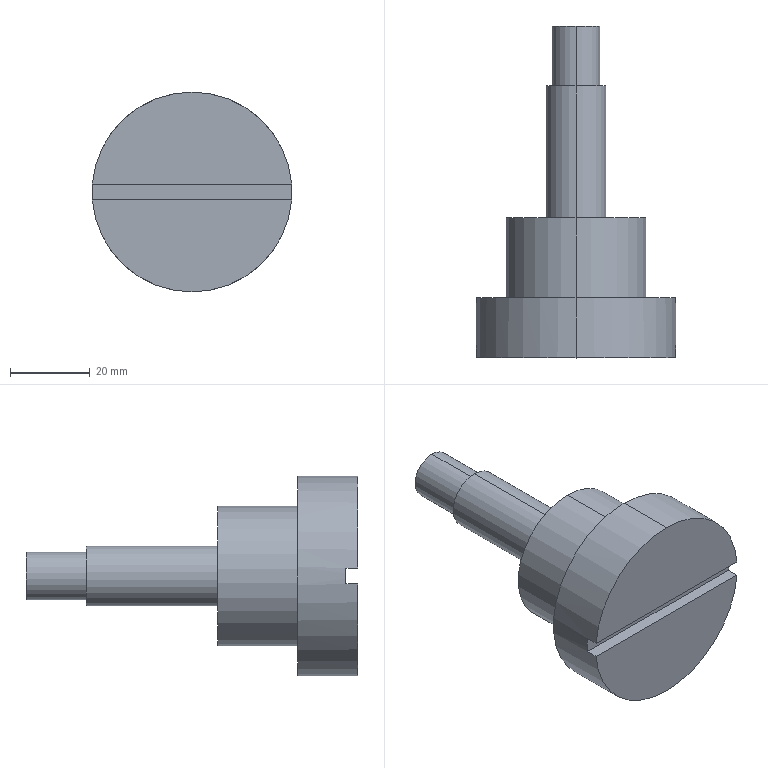Part | STEP file | Large handwheel QY-1-36 | 1 solid | 17 faces | box 50 x 83 x 50 mm | volume 55623 mm3 | plane 9 | cylinder 8 | commonest cylinder face diameters 12 x2 15 x2 35 x2 50 x2
STEP:
#1=CARTESIAN_POINT('',(0.,0.,0.));
#2=DIRECTION('',(0.,0.,1.));
#3=DIRECTION('',(1.,0.,0.));
#4=AXIS2_PLACEMENT_3D('',#1,#2,#3);
#5=CARTESIAN_POINT('',(0.,83.,6.));
#6=VERTEX_POINT('',#5);
#7=CARTESIAN_POINT('',(0.,83.,-6.));
#8=VERTEX_POINT('',#7);
#9=CARTESIAN_POINT('',(0.,83.,0.));
#10=DIRECTION('',(0.,1.,0.));
#11=DIRECTION('',(0.,0.,1.));
#12=AXIS2_PLACEMENT_3D('',#9,#10,#11);
#13=CIRCLE('',#12,6.);
#14=CARTESIAN_POINT('',(0.,83.,0.));
#15=DIRECTION('',(0.,-1.,0.));
#16=DIRECTION('',(0.,0.,-1.));
#17=AXIS2_PLACEMENT_3D('',#14,#15,#16);
#18=CYLINDRICAL_SURFACE('',#17,6.);
#19=CARTESIAN_POINT('',(3.142,0.));
#20=DIRECTION('',(-1.,0.));
#21=VECTOR('',#20,1.);
#22=LINE('',#19,#21);
#23=(GEOMETRIC_REPRESENTATION_CONTEXT(2)PARAMETRIC_REPRESENTATION_CONTEXT()REPRESENTATION_CONTEXT('',''));
#24=DEFINITIONAL_REPRESENTATION('',(#22),#23);
#25=PCURVE('',#18,#24);
#26=CARTESIAN_POINT('',(0.,83.,0.));
#27=DIRECTION('',(0.,1.,0.));
#28=DIRECTION('',(0.,0.,1.));
#29=AXIS2_PLACEMENT_3D('',#26,#27,#28);
#30=PLANE('',#29);
#31=CARTESIAN_POINT('',(0.,0.));
#32=DIRECTION('',(1.,0.));
#33=AXIS2_PLACEMENT_2D('',#31,#32);
#34=CIRCLE('',#33,6.);
#35=(GEOMETRIC_REPRESENTATION_CONTEXT(2)PARAMETRIC_REPRESENTATION_CONTEXT()REPRESENTATION_CONTEXT('',''));
#36=DEFINITIONAL_REPRESENTATION('',(#34),#35);
#37=PCURVE('',#30,#36);
#38=SURFACE_CURVE('',#13,(#25,#37),.PCURVE_S1.);
#39=EDGE_CURVE('',#6,#8,#38,.T.);
#40=ORIENTED_EDGE('',*,*,#39,.F.);
#41=CARTESIAN_POINT('',(0.,68.,6.));
#42=VERTEX_POINT('',#41);
#43=CARTESIAN_POINT('',(0.,83.,6.));
#44=DIRECTION('',(0.,-1.,0.));
#45=VECTOR('',#44,1.);
#46=LINE('',#43,#45);
#47=CARTESIAN_POINT('',(3.142,0.));
#48=DIRECTION('',(0.,1.));
#49=VECTOR('',#48,1.);
#50=LINE('',#47,#49);
#51=(GEOMETRIC_REPRESENTATION_CONTEXT(2)PARAMETRIC_REPRESENTATION_CONTEXT()REPRESENTATION_CONTEXT('',''));
#52=DEFINITIONAL_REPRESENTATION('',(#50),#51);
#53=PCURVE('',#18,#52);
#54=CARTESIAN_POINT('',(0.,83.,0.));
#55=DIRECTION('',(0.,-1.,0.));
#56=DIRECTION('',(0.,0.,-1.));
#57=AXIS2_PLACEMENT_3D('',#54,#55,#56);
#58=CYLINDRICAL_SURFACE('',#57,6.);
#59=CARTESIAN_POINT('',(3.142,0.));
#60=DIRECTION('',(0.,1.));
#61=VECTOR('',#60,1.);
#62=LINE('',#59,#61);
#63=(GEOMETRIC_REPRESENTATION_CONTEXT(2)PARAMETRIC_REPRESENTATION_CONTEXT()REPRESENTATION_CONTEXT('',''));
#64=DEFINITIONAL_REPRESENTATION('',(#62),#63);
#65=PCURVE('',#58,#64);
#66=SURFACE_CURVE('',#46,(#53,#65),.PCURVE_S1.);
#67=EDGE_CURVE('',#6,#42,#66,.T.);
#68=ORIENTED_EDGE('',*,*,#67,.T.);
#69=CARTESIAN_POINT('',(0.,68.,-6.));
#70=VERTEX_POINT('',#69);
#71=CARTESIAN_POINT('',(0.,68.,0.));
#72=DIRECTION('',(0.,1.,0.));
#73=DIRECTION('',(0.,0.,1.));
#74=AXIS2_PLACEMENT_3D('',#71,#72,#73);
#75=CIRCLE('',#74,6.);
#76=CARTESIAN_POINT('',(3.142,15.));
#77=DIRECTION('',(-1.,0.));
#78=VECTOR('',#77,1.);
#79=LINE('',#76,#78);
#80=(GEOMETRIC_REPRESENTATION_CONTEXT(2)PARAMETRIC_REPRESENTATION_CONTEXT()REPRESENTATION_CONTEXT('',''));
#81=DEFINITIONAL_REPRESENTATION('',(#79),#80);
#82=PCURVE('',#18,#81);
#83=CARTESIAN_POINT('',(0.,68.,0.));
#84=DIRECTION('',(0.,1.,0.));
#85=DIRECTION('',(0.,0.,1.));
#86=AXIS2_PLACEMENT_3D('',#83,#84,#85);
#87=PLANE('',#86);
#88=CARTESIAN_POINT('',(0.,0.));
#89=DIRECTION('',(1.,0.));
#90=AXIS2_PLACEMENT_2D('',#88,#89);
#91=CIRCLE('',#90,6.);
#92=(GEOMETRIC_REPRESENTATION_CONTEXT(2)PARAMETRIC_REPRESENTATION_CONTEXT()REPRESENTATION_CONTEXT('',''));
#93=DEFINITIONAL_REPRESENTATION('',(#91),#92);
#94=PCURVE('',#87,#93);
#95=SURFACE_CURVE('',#75,(#82,#94),.PCURVE_S1.);
#96=EDGE_CURVE('',#42,#70,#95,.T.);
#97=ORIENTED_EDGE('',*,*,#96,.T.);
#98=CARTESIAN_POINT('',(0.,83.,-6.));
#99=DIRECTION('',(0.,-1.,0.));
#100=VECTOR('',#99,1.);
#101=LINE('',#98,#100);
#102=CARTESIAN_POINT('',(0.,0.));
#103=DIRECTION('',(0.,1.));
#104=VECTOR('',#103,1.);
#105=LINE('',#102,#104);
#106=(GEOMETRIC_REPRESENTATION_CONTEXT(2)PARAMETRIC_REPRESENTATION_CONTEXT()REPRESENTATION_CONTEXT('',''));
#107=DEFINITIONAL_REPRESENTATION('',(#105),#106);
#108=PCURVE('',#18,#107);
#109=CARTESIAN_POINT('',(6.283,0.));
#110=DIRECTION('',(0.,1.));
#111=VECTOR('',#110,1.);
#112=LINE('',#109,#111);
#113=(GEOMETRIC_REPRESENTATION_CONTEXT(2)PARAMETRIC_REPRESENTATION_CONTEXT()REPRESENTATION_CONTEXT('',''));
#114=DEFINITIONAL_REPRESENTATION('',(#112),#113);
#115=PCURVE('',#58,#114);
#116=SURFACE_CURVE('',#101,(#108,#115),.PCURVE_S1.);
#117=EDGE_CURVE('',#8,#70,#116,.T.);
#118=ORIENTED_EDGE('',*,*,#117,.F.);
#119=EDGE_LOOP('',(#40,#68,#97,#118));
#120=FACE_BOUND('',#119,.T.);
#121=ADVANCED_FACE('',(#120),#18,.T.);
#122=CARTESIAN_POINT('',(0.,68.,7.5));
#123=VERTEX_POINT('',#122);
#124=CARTESIAN_POINT('',(0.,68.,-7.5));
#125=VERTEX_POINT('',#124);
#126=CARTESIAN_POINT('',(0.,68.,0.));
#127=DIRECTION('',(0.,1.,0.));
#128=DIRECTION('',(0.,0.,1.));
#129=AXIS2_PLACEMENT_3D('',#126,#127,#128);
#130=CIRCLE('',#129,7.5);
#131=CARTESIAN_POINT('',(0.,68.,0.));
#132=DIRECTION('',(0.,-1.,0.));
#133=DIRECTION('',(0.,0.,-1.));
#134=AXIS2_PLACEMENT_3D('',#131,#132,#133);
#135=CYLINDRICAL_SURFACE('',#134,7.5);
#136=CARTESIAN_POINT('',(3.142,0.));
#137=DIRECTION('',(-1.,0.));
#138=VECTOR('',#137,1.);
#139=LINE('',#136,#138);
#140=(GEOMETRIC_REPRESENTATION_CONTEXT(2)PARAMETRIC_REPRESENTATION_CONTEXT()REPRESENTATION_CONTEXT('',''));
#141=DEFINITIONAL_REPRESENTATION('',(#139),#140);
#142=PCURVE('',#135,#141);
#143=CARTESIAN_POINT('',(0.,0.));
#144=DIRECTION('',(1.,0.));
#145=AXIS2_PLACEMENT_2D('',#143,#144);
#146=CIRCLE('',#145,7.5);
#147=(GEOMETRIC_REPRESENTATION_CONTEXT(2)PARAMETRIC_REPRESENTATION_CONTEXT()REPRESENTATION_CONTEXT('',''));
#148=DEFINITIONAL_REPRESENTATION('',(#146),#147);
#149=PCURVE('',#87,#148);
#150=SURFACE_CURVE('',#130,(#142,#149),.PCURVE_S1.);
#151=EDGE_CURVE('',#123,#125,#150,.T.);
#152=ORIENTED_EDGE('',*,*,#151,.F.);
#153=CARTESIAN_POINT('',(0.,35.,7.5));
#154=VERTEX_POINT('',#153);
#155=CARTESIAN_POINT('',(0.,68.,7.5));
#156=DIRECTION('',(0.,-1.,0.));
#157=VECTOR('',#156,1.);
#158=LINE('',#155,#157);
#159=CARTESIAN_POINT('',(3.142,0.));
#160=DIRECTION('',(0.,1.));
#161=VECTOR('',#160,1.);
#162=LINE('',#159,#161);
#163=(GEOMETRIC_REPRESENTATION_CONTEXT(2)PARAMETRIC_REPRESENTATION_CONTEXT()REPRESENTATION_CONTEXT('',''));
#164=DEFINITIONAL_REPRESENTATION('',(#162),#163);
#165=PCURVE('',#135,#164);
#166=CARTESIAN_POINT('',(0.,68.,0.));
#167=DIRECTION('',(0.,-1.,0.));
#168=DIRECTION('',(0.,0.,-1.));
#169=AXIS2_PLACEMENT_3D('',#166,#167,#168);
#170=CYLINDRICAL_SURFACE('',#169,7.5);
#171=CARTESIAN_POINT('',(3.142,0.));
#172=DIRECTION('',(0.,1.));
#173=VECTOR('',#172,1.);
#174=LINE('',#171,#173);
#175=(GEOMETRIC_REPRESENTATION_CONTEXT(2)PARAMETRIC_REPRESENTATION_CONTEXT()REPRESENTATION_CONTEXT('',''));
#176=DEFINITIONAL_REPRESENTATION('',(#174),#175);
#177=PCURVE('',#170,#176);
#178=SURFACE_CURVE('',#158,(#165,#177),.PCURVE_S1.);
#179=EDGE_CURVE('',#123,#154,#178,.T.);
#180=ORIENTED_EDGE('',*,*,#179,.T.);
#181=CARTESIAN_POINT('',(0.,35.,-7.5));
#182=VERTEX_POINT('',#181);
#183=CARTESIAN_POINT('',(0.,35.,0.));
#184=DIRECTION('',(0.,1.,0.));
#185=DIRECTION('',(0.,0.,1.));
#186=AXIS2_PLACEMENT_3D('',#183,#184,#185);
#187=CIRCLE('',#186,7.5);
#188=CARTESIAN_POINT('',(3.142,33.));
#189=DIRECTION('',(-1.,0.));
#190=VECTOR('',#189,1.);
#191=LINE('',#188,#190);
#192=(GEOMETRIC_REPRESENTATION_CONTEXT(2)PARAMETRIC_REPRESENTATION_CONTEXT()REPRESENTATION_CONTEXT('',''));
#193=DEFINITIONAL_REPRESENTATION('',(#191),#192);
#194=PCURVE('',#135,#193);
#195=CARTESIAN_POINT('',(0.,35.,0.));
#196=DIRECTION('',(0.,1.,0.));
#197=DIRECTION('',(0.,0.,1.));
#198=AXIS2_PLACEMENT_3D('',#195,#196,#197);
#199=PLANE('',#198);
#200=CARTESIAN_POINT('',(0.,0.));
#201=DIRECTION('',(1.,0.));
#202=AXIS2_PLACEMENT_2D('',#200,#201);
#203=CIRCLE('',#202,7.5);
#204=(GEOMETRIC_REPRESENTATION_CONTEXT(2)PARAMETRIC_REPRESENTATION_CONTEXT()REPRESENTATION_CONTEXT('',''));
#205=DEFINITIONAL_REPRESENTATION('',(#203),#204);
#206=PCURVE('',#199,#205);
#207=SURFACE_CURVE('',#187,(#194,#206),.PCURVE_S1.);
#208=EDGE_CURVE('',#154,#182,#207,.T.);
#209=ORIENTED_EDGE('',*,*,#208,.T.);
#210=CARTESIAN_POINT('',(0.,68.,-7.5));
#211=DIRECTION('',(0.,-1.,0.));
#212=VECTOR('',#211,1.);
#213=LINE('',#210,#212);
#214=CARTESIAN_POINT('',(0.,0.));
#215=DIRECTION('',(0.,1.));
#216=VECTOR('',#215,1.);
#217=LINE('',#214,#216);
#218=(GEOMETRIC_REPRESENTATION_CONTEXT(2)PARAMETRIC_REPRESENTATION_CONTEXT()REPRESENTATION_CONTEXT('',''));
#219=DEFINITIONAL_REPRESENTATION('',(#217),#218);
#220=PCURVE('',#135,#219);
#221=CARTESIAN_POINT('',(6.283,0.));
#222=DIRECTION('',(0.,1.));
#223=VECTOR('',#222,1.);
#224=LINE('',#221,#223);
#225=(GEOMETRIC_REPRESENTATION_CONTEXT(2)PARAMETRIC_REPRESENTATION_CONTEXT()REPRESENTATION_CONTEXT('',''));
#226=DEFINITIONAL_REPRESENTATION('',(#224),#225);
#227=PCURVE('',#170,#226);
#228=SURFACE_CURVE('',#213,(#220,#227),.PCURVE_S1.);
#229=EDGE_CURVE('',#125,#182,#228,.T.);
#230=ORIENTED_EDGE('',*,*,#229,.F.);
#231=EDGE_LOOP('',(#152,#180,#209,#230));
#232=FACE_BOUND('',#231,.T.);
#233=ADVANCED_FACE('',(#232),#135,.T.);
#234=CARTESIAN_POINT('',(0.,35.,17.5));
#235=VERTEX_POINT('',#234);
#236=CARTESIAN_POINT('',(0.,35.,-17.5));
#237=VERTEX_POINT('',#236);
#238=CARTESIAN_POINT('',(0.,35.,0.));
#239=DIRECTION('',(0.,1.,0.));
#240=DIRECTION('',(0.,0.,1.));
#241=AXIS2_PLACEMENT_3D('',#238,#239,#240);
#242=CIRCLE('',#241,17.5);
#243=CARTESIAN_POINT('',(0.,35.,0.));
#244=DIRECTION('',(0.,-1.,0.));
#245=DIRECTION('',(0.,0.,-1.));
#246=AXIS2_PLACEMENT_3D('',#243,#244,#245);
#247=CYLINDRICAL_SURFACE('',#246,17.5);
#248=CARTESIAN_POINT('',(3.142,0.));
#249=DIRECTION('',(-1.,0.));
#250=VECTOR('',#249,1.);
#251=LINE('',#248,#250);
#252=(GEOMETRIC_REPRESENTATION_CONTEXT(2)PARAMETRIC_REPRESENTATION_CONTEXT()REPRESENTATION_CONTEXT('',''));
#253=DEFINITIONAL_REPRESENTATION('',(#251),#252);
#254=PCURVE('',#247,#253);
#255=CARTESIAN_POINT('',(0.,0.));
#256=DIRECTION('',(1.,0.));
#257=AXIS2_PLACEMENT_2D('',#255,#256);
#258=CIRCLE('',#257,17.5);
#259=(GEOMETRIC_REPRESENTATION_CONTEXT(2)PARAMETRIC_REPRESENTATION_CONTEXT()REPRESENTATION_CONTEXT('',''));
#260=DEFINITIONAL_REPRESENTATION('',(#258),#259);
#261=PCURVE('',#199,#260);
#262=SURFACE_CURVE('',#242,(#254,#261),.PCURVE_S1.);
#263=EDGE_CURVE('',#235,#237,#262,.T.);
#264=ORIENTED_EDGE('',*,*,#263,.F.);
#265=CARTESIAN_POINT('',(0.,15.,17.5));
#266=VERTEX_POINT('',#265);
#267=CARTESIAN_POINT('',(0.,35.,17.5));
#268=DIRECTION('',(0.,-1.,0.));
#269=VECTOR('',#268,1.);
#270=LINE('',#267,#269);
#271=CARTESIAN_POINT('',(3.142,0.));
#272=DIRECTION('',(0.,1.));
#273=VECTOR('',#272,1.);
#274=LINE('',#271,#273);
#275=(GEOMETRIC_REPRESENTATION_CONTEXT(2)PARAMETRIC_REPRESENTATION_CONTEXT()REPRESENTATION_CONTEXT('',''));
#276=DEFINITIONAL_REPRESENTATION('',(#274),#275);
#277=PCURVE('',#247,#276);
#278=CARTESIAN_POINT('',(0.,35.,0.));
#279=DIRECTION('',(0.,-1.,0.));
#280=DIRECTION('',(0.,0.,-1.));
#281=AXIS2_PLACEMENT_3D('',#278,#279,#280);
#282=CYLINDRICAL_SURFACE('',#281,17.5);
#283=CARTESIAN_POINT('',(3.142,0.));
#284=DIRECTION('',(0.,1.));
#285=VECTOR('',#284,1.);
#286=LINE('',#283,#285);
#287=(GEOMETRIC_REPRESENTATION_CONTEXT(2)PARAMETRIC_REPRESENTATION_CONTEXT()REPRESENTATION_CONTEXT('',''));
#288=DEFINITIONAL_REPRESENTATION('',(#286),#287);
#289=PCURVE('',#282,#288);
#290=SURFACE_CURVE('',#270,(#277,#289),.PCURVE_S1.);
#291=EDGE_CURVE('',#235,#266,#290,.T.);
#292=ORIENTED_EDGE('',*,*,#291,.T.);
#293=CARTESIAN_POINT('',(0.,15.,-17.5));
#294=VERTEX_POINT('',#293);
#295=CARTESIAN_POINT('',(0.,15.,0.));
#296=DIRECTION('',(0.,1.,0.));
#297=DIRECTION('',(0.,0.,1.));
#298=AXIS2_PLACEMENT_3D('',#295,#296,#297);
#299=CIRCLE('',#298,17.5);
#300=CARTESIAN_POINT('',(3.142,20.));
#301=DIRECTION('',(-1.,0.));
#302=VECTOR('',#301,1.);
#303=LINE('',#300,#302);
#304=(GEOMETRIC_REPRESENTATION_CONTEXT(2)PARAMETRIC_REPRESENTATION_CONTEXT()REPRESENTATION_CONTEXT('',''));
#305=DEFINITIONAL_REPRESENTATION('',(#303),#304);
#306=PCURVE('',#247,#305);
#307=CARTESIAN_POINT('',(0.,15.,0.));
#308=DIRECTION('',(0.,1.,0.));
#309=DIRECTION('',(0.,0.,1.));
#310=AXIS2_PLACEMENT_3D('',#307,#308,#309);
#311=PLANE('',#310);
#312=CARTESIAN_POINT('',(0.,0.));
#313=DIRECTION('',(1.,0.));
#314=AXIS2_PLACEMENT_2D('',#312,#313);
#315=CIRCLE('',#314,17.5);
#316=(GEOMETRIC_REPRESENTATION_CONTEXT(2)PARAMETRIC_REPRESENTATION_CONTEXT()REPRESENTATION_CONTEXT('',''));
#317=DEFINITIONAL_REPRESENTATION('',(#315),#316);
#318=PCURVE('',#311,#317);
#319=SURFACE_CURVE('',#299,(#306,#318),.PCURVE_S1.);
#320=EDGE_CURVE('',#266,#294,#319,.T.);
#321=ORIENTED_EDGE('',*,*,#320,.T.);
#322=CARTESIAN_POINT('',(0.,35.,-17.5));
#323=DIRECTION('',(0.,-1.,0.));
#324=VECTOR('',#323,1.);
#325=LINE('',#322,#324);
#326=CARTESIAN_POINT('',(0.,0.));
#327=DIRECTION('',(0.,1.));
#328=VECTOR('',#327,1.);
#329=LINE('',#326,#328);
#330=(GEOMETRIC_REPRESENTATION_CONTEXT(2)PARAMETRIC_REPRESENTATION_CONTEXT()REPRESENTATION_CONTEXT('',''));
#331=DEFINITIONAL_REPRESENTATION('',(#329),#330);
#332=PCURVE('',#247,#331);
#333=CARTESIAN_POINT('',(6.283,0.));
#334=DIRECTION('',(0.,1.));
#335=VECTOR('',#334,1.);
#336=LINE('',#333,#335);
#337=(GEOMETRIC_REPRESENTATION_CONTEXT(2)PARAMETRIC_REPRESENTATION_CONTEXT()REPRESENTATION_CONTEXT('',''));
#338=DEFINITIONAL_REPRESENTATION('',(#336),#337);
#339=PCURVE('',#282,#338);
#340=SURFACE_CURVE('',#325,(#332,#339),.PCURVE_S1.);
#341=EDGE_CURVE('',#237,#294,#340,.T.);
#342=ORIENTED_EDGE('',*,*,#341,.F.);
#343=EDGE_LOOP('',(#264,#292,#321,#342));
#344=FACE_BOUND('',#343,.T.);
#345=ADVANCED_FACE('',(#344),#247,.T.);
#346=CARTESIAN_POINT('',(0.,15.,25.));
#347=VERTEX_POINT('',#346);
#348=CARTESIAN_POINT('',(0.,15.,-25.));
#349=VERTEX_POINT('',#348);
#350=CARTESIAN_POINT('',(0.,15.,0.));
#351=DIRECTION('',(0.,1.,0.));
#352=DIRECTION('',(0.,0.,1.));
#353=AXIS2_PLACEMENT_3D('',#350,#351,#352);
#354=CIRCLE('',#353,25.);
#355=CARTESIAN_POINT('',(0.,15.,0.));
#356=DIRECTION('',(0.,-1.,0.));
#357=DIRECTION('',(0.,0.,-1.));
#358=AXIS2_PLACEMENT_3D('',#355,#356,#357);
#359=CYLINDRICAL_SURFACE('',#358,25.);
#360=CARTESIAN_POINT('',(3.142,0.));
#361=DIRECTION('',(-1.,0.));
#362=VECTOR('',#361,1.);
#363=LINE('',#360,#362);
#364=(GEOMETRIC_REPRESENTATION_CONTEXT(2)PARAMETRIC_REPRESENTATION_CONTEXT()REPRESENTATION_CONTEXT('',''));
#365=DEFINITIONAL_REPRESENTATION('',(#363),#364);
#366=PCURVE('',#359,#365);
#367=CARTESIAN_POINT('',(0.,0.));
#368=DIRECTION('',(1.,0.));
#369=AXIS2_PLACEMENT_2D('',#367,#368);
#370=CIRCLE('',#369,25.);
#371=(GEOMETRIC_REPRESENTATION_CONTEXT(2)PARAMETRIC_REPRESENTATION_CONTEXT()REPRESENTATION_CONTEXT('',''));
#372=DEFINITIONAL_REPRESENTATION('',(#370),#371);
#373=PCURVE('',#311,#372);
#374=SURFACE_CURVE('',#354,(#366,#373),.PCURVE_S1.);
#375=EDGE_CURVE('',#347,#349,#374,.T.);
#376=ORIENTED_EDGE('',*,*,#375,.F.);
#377=CARTESIAN_POINT('',(0.,0.,25.));
#378=VERTEX_POINT('',#377);
#379=CARTESIAN_POINT('',(0.,15.,25.));
#380=DIRECTION('',(0.,-1.,0.));
#381=VECTOR('',#380,1.);
#382=LINE('',#379,#381);
#383=CARTESIAN_POINT('',(3.142,0.));
#384=DIRECTION('',(0.,1.));
#385=VECTOR('',#384,1.);
#386=LINE('',#383,#385);
#387=(GEOMETRIC_REPRESENTATION_CONTEXT(2)PARAMETRIC_REPRESENTATION_CONTEXT()REPRESENTATION_CONTEXT('',''));
#388=DEFINITIONAL_REPRESENTATION('',(#386),#387);
#389=PCURVE('',#359,#388);
#390=CARTESIAN_POINT('',(0.,15.,0.));
#391=DIRECTION('',(0.,-1.,0.));
#392=DIRECTION('',(0.,0.,-1.));
#393=AXIS2_PLACEMENT_3D('',#390,#391,#392);
#394=CYLINDRICAL_SURFACE('',#393,25.);
#395=CARTESIAN_POINT('',(3.142,0.));
#396=DIRECTION('',(0.,1.));
#397=VECTOR('',#396,1.);
#398=LINE('',#395,#397);
#399=(GEOMETRIC_REPRESENTATION_CONTEXT(2)PARAMETRIC_REPRESENTATION_CONTEXT()REPRESENTATION_CONTEXT('',''));
#400=DEFINITIONAL_REPRESENTATION('',(#398),#399);
#401=PCURVE('',#394,#400);
#402=SURFACE_CURVE('',#382,(#389,#401),.PCURVE_S1.);
#403=EDGE_CURVE('',#347,#378,#402,.T.);
#404=ORIENTED_EDGE('',*,*,#403,.T.);
#405=CARTESIAN_POINT('',(24.92,0.,2.));
#406=VERTEX_POINT('',#405);
#407=CARTESIAN_POINT('',(0.,0.,0.));
#408=DIRECTION('',(0.,1.,0.));
#409=DIRECTION('',(0.,0.,1.));
#410=AXIS2_PLACEMENT_3D('',#407,#408,#409);
#411=CIRCLE('',#410,25.);
#412=CARTESIAN_POINT('',(3.142,15.));
#413=DIRECTION('',(-1.,0.));
#414=VECTOR('',#413,1.);
#415=LINE('',#412,#414);
#416=(GEOMETRIC_REPRESENTATION_CONTEXT(2)PARAMETRIC_REPRESENTATION_CONTEXT()REPRESENTATION_CONTEXT('',''));
#417=DEFINITIONAL_REPRESENTATION('',(#415),#416);
#418=PCURVE('',#359,#417);
#419=CARTESIAN_POINT('',(0.,0.,0.));
#420=DIRECTION('',(0.,1.,0.));
#421=DIRECTION('',(0.,0.,1.));
#422=AXIS2_PLACEMENT_3D('',#419,#420,#421);
#423=PLANE('',#422);
#424=CARTESIAN_POINT('',(0.,0.));
#425=DIRECTION('',(1.,0.));
#426=AXIS2_PLACEMENT_2D('',#424,#425);
#427=CIRCLE('',#426,25.);
#428=(GEOMETRIC_REPRESENTATION_CONTEXT(2)PARAMETRIC_REPRESENTATION_CONTEXT()REPRESENTATION_CONTEXT('',''));
#429=DEFINITIONAL_REPRESENTATION('',(#427),#428);
#430=PCURVE('',#423,#429);
#431=SURFACE_CURVE('',#411,(#418,#430),.PCURVE_S1.);
#432=EDGE_CURVE('',#378,#406,#431,.T.);
#433=ORIENTED_EDGE('',*,*,#432,.T.);
#434=CARTESIAN_POINT('',(24.92,3.,2.));
#435=VERTEX_POINT('',#434);
#436=CARTESIAN_POINT('',(24.92,15.,2.));
#437=DIRECTION('',(0.,1.,0.));
#438=VECTOR('',#437,1.);
#439=LINE('',#436,#438);
#440=CARTESIAN_POINT('',(1.651,0.));
#441=DIRECTION('',(0.,-1.));
#442=VECTOR('',#441,1.);
#443=LINE('',#440,#442);
#444=(GEOMETRIC_REPRESENTATION_CONTEXT(2)PARAMETRIC_REPRESENTATION_CONTEXT()REPRESENTATION_CONTEXT('',''));
#445=DEFINITIONAL_REPRESENTATION('',(#443),#444);
#446=PCURVE('',#359,#445);
#447=CARTESIAN_POINT('',(-71.5,3.,2.));
#448=DIRECTION('',(0.,0.,1.));
#449=DIRECTION('',(1.,0.,0.));
#450=AXIS2_PLACEMENT_3D('',#447,#448,#449);
#451=PLANE('',#450);
#452=CARTESIAN_POINT('',(96.42,12.));
#453=DIRECTION('',(0.,1.));
#454=VECTOR('',#453,1.);
#455=LINE('',#452,#454);
#456=(GEOMETRIC_REPRESENTATION_CONTEXT(2)PARAMETRIC_REPRESENTATION_CONTEXT()REPRESENTATION_CONTEXT('',''));
#457=DEFINITIONAL_REPRESENTATION('',(#455),#456);
#458=PCURVE('',#451,#457);
#459=SURFACE_CURVE('',#439,(#446,#458),.PCURVE_S1.);
#460=EDGE_CURVE('',#406,#435,#459,.T.);
#461=ORIENTED_EDGE('',*,*,#460,.T.);
#462=CARTESIAN_POINT('',(24.92,3.,-2.));
#463=VERTEX_POINT('',#462);
#464=CARTESIAN_POINT('',(0.,3.,0.));
#465=DIRECTION('',(0.,1.,0.));
#466=DIRECTION('',(0.,0.,1.));
#467=AXIS2_PLACEMENT_3D('',#464,#465,#466);
#468=CIRCLE('',#467,25.);
#469=CARTESIAN_POINT('',(3.142,12.));
#470=DIRECTION('',(-1.,0.));
#471=VECTOR('',#470,1.);
#472=LINE('',#469,#471);
#473=(GEOMETRIC_REPRESENTATION_CONTEXT(2)PARAMETRIC_REPRESENTATION_CONTEXT()REPRESENTATION_CONTEXT('',''));
#474=DEFINITIONAL_REPRESENTATION('',(#472),#473);
#475=PCURVE('',#359,#474);
#476=CARTESIAN_POINT('',(-71.5,3.,2.));
#477=DIRECTION('',(0.,1.,0.));
#478=DIRECTION('',(0.,0.,1.));
#479=AXIS2_PLACEMENT_3D('',#476,#477,#478);
#480=PLANE('',#479);
#481=CARTESIAN_POINT('',(-2.,71.5));
#482=DIRECTION('',(1.,0.));
#483=AXIS2_PLACEMENT_2D('',#481,#482);
#484=CIRCLE('',#483,25.);
#485=(GEOMETRIC_REPRESENTATION_CONTEXT(2)PARAMETRIC_REPRESENTATION_CONTEXT()REPRESENTATION_CONTEXT('',''));
#486=DEFINITIONAL_REPRESENTATION('',(#484),#485);
#487=PCURVE('',#480,#486);
#488=SURFACE_CURVE('',#468,(#475,#487),.PCURVE_S1.);
#489=EDGE_CURVE('',#435,#463,#488,.T.);
#490=ORIENTED_EDGE('',*,*,#489,.T.);
#491=CARTESIAN_POINT('',(24.92,0.,-2.));
#492=VERTEX_POINT('',#491);
#493=CARTESIAN_POINT('',(24.92,15.,-2.));
#494=DIRECTION('',(0.,-1.,0.));
#495=VECTOR('',#494,1.);
#496=LINE('',#493,#495);
#497=CARTESIAN_POINT('',(1.491,0.));
#498=DIRECTION('',(0.,1.));
#499=VECTOR('',#498,1.);
#500=LINE('',#497,#499);
#501=(GEOMETRIC_REPRESENTATION_CONTEXT(2)PARAMETRIC_REPRESENTATION_CONTEXT()REPRESENTATION_CONTEXT('',''));
#502=DEFINITIONAL_REPRESENTATION('',(#500),#501);
#503=PCURVE('',#359,#502);
#504=CARTESIAN_POINT('',(-71.5,3.,-2.));
#505=DIRECTION('',(0.,0.,-1.));
#506=DIRECTION('',(-1.,0.,0.));
#507=AXIS2_PLACEMENT_3D('',#504,#505,#506);
#508=PLANE('',#507);
#509=CARTESIAN_POINT('',(-96.42,12.));
#510=DIRECTION('',(0.,-1.));
#511=VECTOR('',#510,1.);
#512=LINE('',#509,#511);
#513=(GEOMETRIC_REPRESENTATION_CONTEXT(2)PARAMETRIC_REPRESENTATION_CONTEXT()REPRESENTATION_CONTEXT('',''));
#514=DEFINITIONAL_REPRESENTATION('',(#512),#513);
#515=PCURVE('',#508,#514);
#516=SURFACE_CURVE('',#496,(#503,#515),.PCURVE_S1.);
#517=EDGE_CURVE('',#463,#492,#516,.T.);
#518=ORIENTED_EDGE('',*,*,#517,.T.);
#519=CARTESIAN_POINT('',(0.,0.,-25.));
#520=VERTEX_POINT('',#519);
#521=CARTESIAN_POINT('',(0.,0.,0.));
#522=DIRECTION('',(0.,1.,0.));
#523=DIRECTION('',(0.,0.,1.));
#524=AXIS2_PLACEMENT_3D('',#521,#522,#523);
#525=CIRCLE('',#524,25.);
#526=CARTESIAN_POINT('',(3.142,15.));
#527=DIRECTION('',(-1.,0.));
#528=VECTOR('',#527,1.);
#529=LINE('',#526,#528);
#530=(GEOMETRIC_REPRESENTATION_CONTEXT(2)PARAMETRIC_REPRESENTATION_CONTEXT()REPRESENTATION_CONTEXT('',''));
#531=DEFINITIONAL_REPRESENTATION('',(#529),#530);
#532=PCURVE('',#359,#531);
#533=CARTESIAN_POINT('',(0.,0.,0.));
#534=DIRECTION('',(0.,1.,0.));
#535=DIRECTION('',(0.,0.,1.));
#536=AXIS2_PLACEMENT_3D('',#533,#534,#535);
#537=PLANE('',#536);
#538=CARTESIAN_POINT('',(0.,0.));
#539=DIRECTION('',(1.,0.));
#540=AXIS2_PLACEMENT_2D('',#538,#539);
#541=CIRCLE('',#540,25.);
#542=(GEOMETRIC_REPRESENTATION_CONTEXT(2)PARAMETRIC_REPRESENTATION_CONTEXT()REPRESENTATION_CONTEXT('',''));
#543=DEFINITIONAL_REPRESENTATION('',(#541),#542);
#544=PCURVE('',#537,#543);
#545=SURFACE_CURVE('',#525,(#532,#544),.PCURVE_S1.);
#546=EDGE_CURVE('',#492,#520,#545,.T.);
#547=ORIENTED_EDGE('',*,*,#546,.T.);
#548=CARTESIAN_POINT('',(0.,15.,-25.));
#549=DIRECTION('',(0.,-1.,0.));
#550=VECTOR('',#549,1.);
#551=LINE('',#548,#550);
#552=CARTESIAN_POINT('',(0.,0.));
#553=DIRECTION('',(0.,1.));
#554=VECTOR('',#553,1.);
#555=LINE('',#552,#554);
#556=(GEOMETRIC_REPRESENTATION_CONTEXT(2)PARAMETRIC_REPRESENTATION_CONTEXT()REPRESENTATION_CONTEXT('',''));
#557=DEFINITIONAL_REPRESENTATION('',(#555),#556);
#558=PCURVE('',#359,#557);
#559=CARTESIAN_POINT('',(6.283,0.));
#560=DIRECTION('',(0.,1.));
#561=VECTOR('',#560,1.);
#562=LINE('',#559,#561);
#563=(GEOMETRIC_REPRESENTATION_CONTEXT(2)PARAMETRIC_REPRESENTATION_CONTEXT()REPRESENTATION_CONTEXT('',''));
#564=DEFINITIONAL_REPRESENTATION('',(#562),#563);
#565=PCURVE('',#394,#564);
#566=SURFACE_CURVE('',#551,(#558,#565),.PCURVE_S1.);
#567=EDGE_CURVE('',#349,#520,#566,.T.);
#568=ORIENTED_EDGE('',*,*,#567,.F.);
#569=EDGE_LOOP('',(#376,#404,#433,#461,#490,#518,#547,#568));
#570=FACE_BOUND('',#569,.T.);
#571=ADVANCED_FACE('',(#570),#359,.T.);
#572=ORIENTED_EDGE('',*,*,#546,.F.);
#573=CARTESIAN_POINT('',(-24.92,0.,-2.));
#574=VERTEX_POINT('',#573);
#575=CARTESIAN_POINT('',(0.,0.,-2.));
#576=DIRECTION('',(-1.,0.,0.));
#577=VECTOR('',#576,1.);
#578=LINE('',#575,#577);
#579=CARTESIAN_POINT('',(-2.,0.));
#580=DIRECTION('',(0.,-1.));
#581=VECTOR('',#580,1.);
#582=LINE('',#579,#581);
#583=(GEOMETRIC_REPRESENTATION_CONTEXT(2)PARAMETRIC_REPRESENTATION_CONTEXT()REPRESENTATION_CONTEXT('',''));
#584=DEFINITIONAL_REPRESENTATION('',(#582),#583);
#585=PCURVE('',#537,#584);
#586=CARTESIAN_POINT('',(-71.5,-3.));
#587=DIRECTION('',(1.,0.));
#588=VECTOR('',#587,1.);
#589=LINE('',#586,#588);
#590=(GEOMETRIC_REPRESENTATION_CONTEXT(2)PARAMETRIC_REPRESENTATION_CONTEXT()REPRESENTATION_CONTEXT('',''));
#591=DEFINITIONAL_REPRESENTATION('',(#589),#590);
#592=PCURVE('',#508,#591);
#593=SURFACE_CURVE('',#578,(#585,#592),.PCURVE_S1.);
#594=EDGE_CURVE('',#492,#574,#593,.T.);
#595=ORIENTED_EDGE('',*,*,#594,.T.);
#596=CARTESIAN_POINT('',(0.,0.,0.));
#597=DIRECTION('',(0.,1.,0.));
#598=DIRECTION('',(0.,0.,1.));
#599=AXIS2_PLACEMENT_3D('',#596,#597,#598);
#600=CIRCLE('',#599,25.);
#601=CARTESIAN_POINT('',(0.,0.));
#602=DIRECTION('',(1.,0.));
#603=AXIS2_PLACEMENT_2D('',#601,#602);
#604=CIRCLE('',#603,25.);
#605=(GEOMETRIC_REPRESENTATION_CONTEXT(2)PARAMETRIC_REPRESENTATION_CONTEXT()REPRESENTATION_CONTEXT('',''));
#606=DEFINITIONAL_REPRESENTATION('',(#604),#605);
#607=PCURVE('',#537,#606);
#608=CARTESIAN_POINT('',(9.425,15.));
#609=DIRECTION('',(-1.,0.));
#610=VECTOR('',#609,1.);
#611=LINE('',#608,#610);
#612=(GEOMETRIC_REPRESENTATION_CONTEXT(2)PARAMETRIC_REPRESENTATION_CONTEXT()REPRESENTATION_CONTEXT('',''));
#613=DEFINITIONAL_REPRESENTATION('',(#611),#612);
#614=PCURVE('',#394,#613);
#615=SURFACE_CURVE('',#600,(#607,#614),.PCURVE_S1.);
#616=EDGE_CURVE('',#520,#574,#615,.T.);
#617=ORIENTED_EDGE('',*,*,#616,.F.);
#618=EDGE_LOOP('',(#572,#595,#617));
#619=FACE_BOUND('',#618,.T.);
#620=ADVANCED_FACE('',(#619),#537,.F.);
#621=ORIENTED_EDGE('',*,*,#403,.F.);
#622=CARTESIAN_POINT('',(0.,15.,0.));
#623=DIRECTION('',(0.,1.,0.));
#624=DIRECTION('',(0.,0.,1.));
#625=AXIS2_PLACEMENT_3D('',#622,#623,#624);
#626=CIRCLE('',#625,25.);
#627=CARTESIAN_POINT('',(9.425,0.));
#628=DIRECTION('',(-1.,0.));
#629=VECTOR('',#628,1.);
#630=LINE('',#627,#629);
#631=(GEOMETRIC_REPRESENTATION_CONTEXT(2)PARAMETRIC_REPRESENTATION_CONTEXT()REPRESENTATION_CONTEXT('',''));
#632=DEFINITIONAL_REPRESENTATION('',(#630),#631);
#633=PCURVE('',#394,#632);
#634=CARTESIAN_POINT('',(0.,0.));
#635=DIRECTION('',(1.,0.));
#636=AXIS2_PLACEMENT_2D('',#634,#635);
#637=CIRCLE('',#636,25.);
#638=(GEOMETRIC_REPRESENTATION_CONTEXT(2)PARAMETRIC_REPRESENTATION_CONTEXT()REPRESENTATION_CONTEXT('',''));
#639=DEFINITIONAL_REPRESENTATION('',(#637),#638);
#640=PCURVE('',#311,#639);
#641=SURFACE_CURVE('',#626,(#633,#640),.PCURVE_S1.);
#642=EDGE_CURVE('',#349,#347,#641,.T.);
#643=ORIENTED_EDGE('',*,*,#642,.F.);
#644=ORIENTED_EDGE('',*,*,#567,.T.);
#645=ORIENTED_EDGE('',*,*,#616,.T.);
#646=CARTESIAN_POINT('',(-24.92,3.,-2.));
#647=VERTEX_POINT('',#646);
#648=CARTESIAN_POINT('',(-24.92,15.,-2.));
#649=DIRECTION('',(0.,1.,0.));
#650=VECTOR('',#649,1.);
#651=LINE('',#648,#650);
#652=CARTESIAN_POINT('',(4.792,0.));
#653=DIRECTION('',(0.,-1.));
#654=VECTOR('',#653,1.);
#655=LINE('',#652,#654);
#656=(GEOMETRIC_REPRESENTATION_CONTEXT(2)PARAMETRIC_REPRESENTATION_CONTEXT()REPRESENTATION_CONTEXT('',''));
#657=DEFINITIONAL_REPRESENTATION('',(#655),#656);
#658=PCURVE('',#394,#657);
#659=CARTESIAN_POINT('',(-46.58,12.));
#660=DIRECTION('',(0.,1.));
#661=VECTOR('',#660,1.);
#662=LINE('',#659,#661);
#663=(GEOMETRIC_REPRESENTATION_CONTEXT(2)PARAMETRIC_REPRESENTATION_CONTEXT()REPRESENTATION_CONTEXT('',''));
#664=DEFINITIONAL_REPRESENTATION('',(#662),#663);
#665=PCURVE('',#508,#664);
#666=SURFACE_CURVE('',#651,(#658,#665),.PCURVE_S1.);
#667=EDGE_CURVE('',#574,#647,#666,.T.);
#668=ORIENTED_EDGE('',*,*,#667,.T.);
#669=CARTESIAN_POINT('',(-24.92,3.,2.));
#670=VERTEX_POINT('',#669);
#671=CARTESIAN_POINT('',(0.,3.,0.));
#672=DIRECTION('',(0.,1.,0.));
#673=DIRECTION('',(0.,0.,1.));
#674=AXIS2_PLACEMENT_3D('',#671,#672,#673);
#675=CIRCLE('',#674,25.);
#676=CARTESIAN_POINT('',(9.425,12.));
#677=DIRECTION('',(-1.,0.));
#678=VECTOR('',#677,1.);
#679=LINE('',#676,#678);
#680=(GEOMETRIC_REPRESENTATION_CONTEXT(2)PARAMETRIC_REPRESENTATION_CONTEXT()REPRESENTATION_CONTEXT('',''));
#681=DEFINITIONAL_REPRESENTATION('',(#679),#680);
#682=PCURVE('',#394,#681);
#683=CARTESIAN_POINT('',(-2.,71.5));
#684=DIRECTION('',(1.,0.));
#685=AXIS2_PLACEMENT_2D('',#683,#684);
#686=CIRCLE('',#685,25.);
#687=(GEOMETRIC_REPRESENTATION_CONTEXT(2)PARAMETRIC_REPRESENTATION_CONTEXT()REPRESENTATION_CONTEXT('',''));
#688=DEFINITIONAL_REPRESENTATION('',(#686),#687);
#689=PCURVE('',#480,#688);
#690=SURFACE_CURVE('',#675,(#682,#689),.PCURVE_S1.);
#691=EDGE_CURVE('',#647,#670,#690,.T.);
#692=ORIENTED_EDGE('',*,*,#691,.T.);
#693=CARTESIAN_POINT('',(-24.92,0.,2.));
#694=VERTEX_POINT('',#693);
#695=CARTESIAN_POINT('',(-24.92,15.,2.));
#696=DIRECTION('',(0.,-1.,0.));
#697=VECTOR('',#696,1.);
#698=LINE('',#695,#697);
#699=CARTESIAN_POINT('',(4.632,0.));
#700=DIRECTION('',(0.,1.));
#701=VECTOR('',#700,1.);
#702=LINE('',#699,#701);
#703=(GEOMETRIC_REPRESENTATION_CONTEXT(2)PARAMETRIC_REPRESENTATION_CONTEXT()REPRESENTATION_CONTEXT('',''));
#704=DEFINITIONAL_REPRESENTATION('',(#702),#703);
#705=PCURVE('',#394,#704);
#706=CARTESIAN_POINT('',(46.58,12.));
#707=DIRECTION('',(0.,-1.));
#708=VECTOR('',#707,1.);
#709=LINE('',#706,#708);
#710=(GEOMETRIC_REPRESENTATION_CONTEXT(2)PARAMETRIC_REPRESENTATION_CONTEXT()REPRESENTATION_CONTEXT('',''));
#711=DEFINITIONAL_REPRESENTATION('',(#709),#710);
#712=PCURVE('',#451,#711);
#713=SURFACE_CURVE('',#698,(#705,#712),.PCURVE_S1.);
#714=EDGE_CURVE('',#670,#694,#713,.T.);
#715=ORIENTED_EDGE('',*,*,#714,.T.);
#716=CARTESIAN_POINT('',(0.,0.,0.));
#717=DIRECTION('',(0.,1.,0.));
#718=DIRECTION('',(0.,0.,1.));
#719=AXIS2_PLACEMENT_3D('',#716,#717,#718);
#720=CIRCLE('',#719,25.);
#721=CARTESIAN_POINT('',(9.425,15.));
#722=DIRECTION('',(-1.,0.));
#723=VECTOR('',#722,1.);
#724=LINE('',#721,#723);
#725=(GEOMETRIC_REPRESENTATION_CONTEXT(2)PARAMETRIC_REPRESENTATION_CONTEXT()REPRESENTATION_CONTEXT('',''));
#726=DEFINITIONAL_REPRESENTATION('',(#724),#725);
#727=PCURVE('',#394,#726);
#728=CARTESIAN_POINT('',(0.,0.));
#729=DIRECTION('',(1.,0.));
#730=AXIS2_PLACEMENT_2D('',#728,#729);
#731=CIRCLE('',#730,25.);
#732=(GEOMETRIC_REPRESENTATION_CONTEXT(2)PARAMETRIC_REPRESENTATION_CONTEXT()REPRESENTATION_CONTEXT('',''));
#733=DEFINITIONAL_REPRESENTATION('',(#731),#732);
#734=PCURVE('',#423,#733);
#735=SURFACE_CURVE('',#720,(#727,#734),.PCURVE_S1.);
#736=EDGE_CURVE('',#694,#378,#735,.T.);
#737=ORIENTED_EDGE('',*,*,#736,.T.);
#738=EDGE_LOOP('',(#621,#643,#644,#645,#668,#692,#715,#737));
#739=FACE_BOUND('',#738,.T.);
#740=ADVANCED_FACE('',(#739),#394,.T.);
#741=CARTESIAN_POINT('',(0.,15.,0.));
#742=DIRECTION('',(0.,1.,0.));
#743=DIRECTION('',(0.,0.,1.));
#744=AXIS2_PLACEMENT_3D('',#741,#742,#743);
#745=CIRCLE('',#744,17.5);
#746=CARTESIAN_POINT('',(0.,0.));
#747=DIRECTION('',(1.,0.));
#748=AXIS2_PLACEMENT_2D('',#746,#747);
#749=CIRCLE('',#748,17.5);
#750=(GEOMETRIC_REPRESENTATION_CONTEXT(2)PARAMETRIC_REPRESENTATION_CONTEXT()REPRESENTATION_CONTEXT('',''));
#751=DEFINITIONAL_REPRESENTATION('',(#749),#750);
#752=PCURVE('',#311,#751);
#753=CARTESIAN_POINT('',(9.425,20.));
#754=DIRECTION('',(-1.,0.));
#755=VECTOR('',#754,1.);
#756=LINE('',#753,#755);
#757=(GEOMETRIC_REPRESENTATION_CONTEXT(2)PARAMETRIC_REPRESENTATION_CONTEXT()REPRESENTATION_CONTEXT('',''));
#758=DEFINITIONAL_REPRESENTATION('',(#756),#757);
#759=PCURVE('',#282,#758);
#760=SURFACE_CURVE('',#745,(#752,#759),.PCURVE_S1.);
#761=EDGE_CURVE('',#294,#266,#760,.T.);
#762=ORIENTED_EDGE('',*,*,#761,.F.);
#763=ORIENTED_EDGE('',*,*,#320,.F.);
#764=EDGE_LOOP('',(#762,#763));
#765=FACE_BOUND('',#764,.T.);
#766=ORIENTED_EDGE('',*,*,#642,.T.);
#767=ORIENTED_EDGE('',*,*,#375,.T.);
#768=EDGE_LOOP('',(#766,#767));
#769=FACE_BOUND('',#768,.T.);
#770=ADVANCED_FACE('',(#765,#769),#311,.T.);
#771=ORIENTED_EDGE('',*,*,#736,.F.);
#772=CARTESIAN_POINT('',(0.,0.,2.));
#773=DIRECTION('',(1.,0.,0.));
#774=VECTOR('',#773,1.);
#775=LINE('',#772,#774);
#776=CARTESIAN_POINT('',(2.,0.));
#777=DIRECTION('',(0.,1.));
#778=VECTOR('',#777,1.);
#779=LINE('',#776,#778);
#780=(GEOMETRIC_REPRESENTATION_CONTEXT(2)PARAMETRIC_REPRESENTATION_CONTEXT()REPRESENTATION_CONTEXT('',''));
#781=DEFINITIONAL_REPRESENTATION('',(#779),#780);
#782=PCURVE('',#423,#781);
#783=CARTESIAN_POINT('',(71.5,-3.));
#784=DIRECTION('',(1.,0.));
#785=VECTOR('',#784,1.);
#786=LINE('',#783,#785);
#787=(GEOMETRIC_REPRESENTATION_CONTEXT(2)PARAMETRIC_REPRESENTATION_CONTEXT()REPRESENTATION_CONTEXT('',''));
#788=DEFINITIONAL_REPRESENTATION('',(#786),#787);
#789=PCURVE('',#451,#788);
#790=SURFACE_CURVE('',#775,(#782,#789),.PCURVE_S1.);
#791=EDGE_CURVE('',#694,#406,#790,.T.);
#792=ORIENTED_EDGE('',*,*,#791,.T.);
#793=ORIENTED_EDGE('',*,*,#432,.F.);
#794=EDGE_LOOP('',(#771,#792,#793));
#795=FACE_BOUND('',#794,.T.);
#796=ADVANCED_FACE('',(#795),#423,.F.);
#797=ORIENTED_EDGE('',*,*,#291,.F.);
#798=CARTESIAN_POINT('',(0.,35.,0.));
#799=DIRECTION('',(0.,1.,0.));
#800=DIRECTION('',(0.,0.,1.));
#801=AXIS2_PLACEMENT_3D('',#798,#799,#800);
#802=CIRCLE('',#801,17.5);
#803=CARTESIAN_POINT('',(9.425,0.));
#804=DIRECTION('',(-1.,0.));
#805=VECTOR('',#804,1.);
#806=LINE('',#803,#805);
#807=(GEOMETRIC_REPRESENTATION_CONTEXT(2)PARAMETRIC_REPRESENTATION_CONTEXT()REPRESENTATION_CONTEXT('',''));
#808=DEFINITIONAL_REPRESENTATION('',(#806),#807);
#809=PCURVE('',#282,#808);
#810=CARTESIAN_POINT('',(0.,0.));
#811=DIRECTION('',(1.,0.));
#812=AXIS2_PLACEMENT_2D('',#810,#811);
#813=CIRCLE('',#812,17.5);
#814=(GEOMETRIC_REPRESENTATION_CONTEXT(2)PARAMETRIC_REPRESENTATION_CONTEXT()REPRESENTATION_CONTEXT('',''));
#815=DEFINITIONAL_REPRESENTATION('',(#813),#814);
#816=PCURVE('',#199,#815);
#817=SURFACE_CURVE('',#802,(#809,#816),.PCURVE_S1.);
#818=EDGE_CURVE('',#237,#235,#817,.T.);
#819=ORIENTED_EDGE('',*,*,#818,.F.);
#820=ORIENTED_EDGE('',*,*,#341,.T.);
#821=ORIENTED_EDGE('',*,*,#761,.T.);
#822=EDGE_LOOP('',(#797,#819,#820,#821));
#823=FACE_BOUND('',#822,.T.);
#824=ADVANCED_FACE('',(#823),#282,.T.);
#825=CARTESIAN_POINT('',(0.,35.,0.));
#826=DIRECTION('',(0.,1.,0.));
#827=DIRECTION('',(0.,0.,1.));
#828=AXIS2_PLACEMENT_3D('',#825,#826,#827);
#829=CIRCLE('',#828,7.5);
#830=CARTESIAN_POINT('',(0.,0.));
#831=DIRECTION('',(1.,0.));
#832=AXIS2_PLACEMENT_2D('',#830,#831);
#833=CIRCLE('',#832,7.5);
#834=(GEOMETRIC_REPRESENTATION_CONTEXT(2)PARAMETRIC_REPRESENTATION_CONTEXT()REPRESENTATION_CONTEXT('',''));
#835=DEFINITIONAL_REPRESENTATION('',(#833),#834);
#836=PCURVE('',#199,#835);
#837=CARTESIAN_POINT('',(9.425,33.));
#838=DIRECTION('',(-1.,0.));
#839=VECTOR('',#838,1.);
#840=LINE('',#837,#839);
#841=(GEOMETRIC_REPRESENTATION_CONTEXT(2)PARAMETRIC_REPRESENTATION_CONTEXT()REPRESENTATION_CONTEXT('',''));
#842=DEFINITIONAL_REPRESENTATION('',(#840),#841);
#843=PCURVE('',#170,#842);
#844=SURFACE_CURVE('',#829,(#836,#843),.PCURVE_S1.);
#845=EDGE_CURVE('',#182,#154,#844,.T.);
#846=ORIENTED_EDGE('',*,*,#845,.F.);
#847=ORIENTED_EDGE('',*,*,#208,.F.);
#848=EDGE_LOOP('',(#846,#847));
#849=FACE_BOUND('',#848,.T.);
#850=ORIENTED_EDGE('',*,*,#818,.T.);
#851=ORIENTED_EDGE('',*,*,#263,.T.);
#852=EDGE_LOOP('',(#850,#851));
#853=FACE_BOUND('',#852,.T.);
#854=ADVANCED_FACE('',(#849,#853),#199,.T.);
#855=ORIENTED_EDGE('',*,*,#179,.F.);
#856=CARTESIAN_POINT('',(0.,68.,0.));
#857=DIRECTION('',(0.,1.,0.));
#858=DIRECTION('',(0.,0.,1.));
#859=AXIS2_PLACEMENT_3D('',#856,#857,#858);
#860=CIRCLE('',#859,7.5);
#861=CARTESIAN_POINT('',(9.425,0.));
#862=DIRECTION('',(-1.,0.));
#863=VECTOR('',#862,1.);
#864=LINE('',#861,#863);
#865=(GEOMETRIC_REPRESENTATION_CONTEXT(2)PARAMETRIC_REPRESENTATION_CONTEXT()REPRESENTATION_CONTEXT('',''));
#866=DEFINITIONAL_REPRESENTATION('',(#864),#865);
#867=PCURVE('',#170,#866);
#868=CARTESIAN_POINT('',(0.,0.));
#869=DIRECTION('',(1.,0.));
#870=AXIS2_PLACEMENT_2D('',#868,#869);
#871=CIRCLE('',#870,7.5);
#872=(GEOMETRIC_REPRESENTATION_CONTEXT(2)PARAMETRIC_REPRESENTATION_CONTEXT()REPRESENTATION_CONTEXT('',''));
#873=DEFINITIONAL_REPRESENTATION('',(#871),#872);
#874=PCURVE('',#87,#873);
#875=SURFACE_CURVE('',#860,(#867,#874),.PCURVE_S1.);
#876=EDGE_CURVE('',#125,#123,#875,.T.);
#877=ORIENTED_EDGE('',*,*,#876,.F.);
#878=ORIENTED_EDGE('',*,*,#229,.T.);
#879=ORIENTED_EDGE('',*,*,#845,.T.);
#880=EDGE_LOOP('',(#855,#877,#878,#879));
#881=FACE_BOUND('',#880,.T.);
#882=ADVANCED_FACE('',(#881),#170,.T.);
#883=CARTESIAN_POINT('',(0.,68.,0.));
#884=DIRECTION('',(0.,1.,0.));
#885=DIRECTION('',(0.,0.,1.));
#886=AXIS2_PLACEMENT_3D('',#883,#884,#885);
#887=CIRCLE('',#886,6.);
#888=CARTESIAN_POINT('',(0.,0.));
#889=DIRECTION('',(1.,0.));
#890=AXIS2_PLACEMENT_2D('',#888,#889);
#891=CIRCLE('',#890,6.);
#892=(GEOMETRIC_REPRESENTATION_CONTEXT(2)PARAMETRIC_REPRESENTATION_CONTEXT()REPRESENTATION_CONTEXT('',''));
#893=DEFINITIONAL_REPRESENTATION('',(#891),#892);
#894=PCURVE('',#87,#893);
#895=CARTESIAN_POINT('',(9.425,15.));
#896=DIRECTION('',(-1.,0.));
#897=VECTOR('',#896,1.);
#898=LINE('',#895,#897);
#899=(GEOMETRIC_REPRESENTATION_CONTEXT(2)PARAMETRIC_REPRESENTATION_CONTEXT()REPRESENTATION_CONTEXT('',''));
#900=DEFINITIONAL_REPRESENTATION('',(#898),#899);
#901=PCURVE('',#58,#900);
#902=SURFACE_CURVE('',#887,(#894,#901),.PCURVE_S1.);
#903=EDGE_CURVE('',#70,#42,#902,.T.);
#904=ORIENTED_EDGE('',*,*,#903,.F.);
#905=ORIENTED_EDGE('',*,*,#96,.F.);
#906=EDGE_LOOP('',(#904,#905));
#907=FACE_BOUND('',#906,.T.);
#908=ORIENTED_EDGE('',*,*,#876,.T.);
#909=ORIENTED_EDGE('',*,*,#151,.T.);
#910=EDGE_LOOP('',(#908,#909));
#911=FACE_BOUND('',#910,.T.);
#912=ADVANCED_FACE('',(#907,#911),#87,.T.);
#913=ORIENTED_EDGE('',*,*,#67,.F.);
#914=CARTESIAN_POINT('',(0.,83.,0.));
#915=DIRECTION('',(0.,1.,0.));
#916=DIRECTION('',(0.,0.,1.));
#917=AXIS2_PLACEMENT_3D('',#914,#915,#916);
#918=CIRCLE('',#917,6.);
#919=CARTESIAN_POINT('',(9.425,0.));
#920=DIRECTION('',(-1.,0.));
#921=VECTOR('',#920,1.);
#922=LINE('',#919,#921);
#923=(GEOMETRIC_REPRESENTATION_CONTEXT(2)PARAMETRIC_REPRESENTATION_CONTEXT()REPRESENTATION_CONTEXT('',''));
#924=DEFINITIONAL_REPRESENTATION('',(#922),#923);
#925=PCURVE('',#58,#924);
#926=CARTESIAN_POINT('',(0.,0.));
#927=DIRECTION('',(1.,0.));
#928=AXIS2_PLACEMENT_2D('',#926,#927);
#929=CIRCLE('',#928,6.);
#930=(GEOMETRIC_REPRESENTATION_CONTEXT(2)PARAMETRIC_REPRESENTATION_CONTEXT()REPRESENTATION_CONTEXT('',''));
#931=DEFINITIONAL_REPRESENTATION('',(#929),#930);
#932=PCURVE('',#30,#931);
#933=SURFACE_CURVE('',#918,(#925,#932),.PCURVE_S1.);
#934=EDGE_CURVE('',#8,#6,#933,.T.);
#935=ORIENTED_EDGE('',*,*,#934,.F.);
#936=ORIENTED_EDGE('',*,*,#117,.T.);
#937=ORIENTED_EDGE('',*,*,#903,.T.);
#938=EDGE_LOOP('',(#913,#935,#936,#937));
#939=FACE_BOUND('',#938,.T.);
#940=ADVANCED_FACE('',(#939),#58,.T.);
#941=ORIENTED_EDGE('',*,*,#934,.T.);
#942=ORIENTED_EDGE('',*,*,#39,.T.);
#943=EDGE_LOOP('',(#941,#942));
#944=FACE_BOUND('',#943,.T.);
#945=ADVANCED_FACE('',(#944),#30,.T.);
#946=CARTESIAN_POINT('',(-71.5,3.,2.));
#947=DIRECTION('',(1.,0.,0.));
#948=VECTOR('',#947,1.);
#949=LINE('',#946,#948);
#950=CARTESIAN_POINT('',(0.,0.));
#951=DIRECTION('',(0.,1.));
#952=VECTOR('',#951,1.);
#953=LINE('',#950,#952);
#954=(GEOMETRIC_REPRESENTATION_CONTEXT(2)PARAMETRIC_REPRESENTATION_CONTEXT()REPRESENTATION_CONTEXT('',''));
#955=DEFINITIONAL_REPRESENTATION('',(#953),#954);
#956=PCURVE('',#480,#955);
#957=CARTESIAN_POINT('',(0.,0.));
#958=DIRECTION('',(1.,0.));
#959=VECTOR('',#958,1.);
#960=LINE('',#957,#959);
#961=(GEOMETRIC_REPRESENTATION_CONTEXT(2)PARAMETRIC_REPRESENTATION_CONTEXT()REPRESENTATION_CONTEXT('',''));
#962=DEFINITIONAL_REPRESENTATION('',(#960),#961);
#963=PCURVE('',#451,#962);
#964=SURFACE_CURVE('',#949,(#956,#963),.PCURVE_S1.);
#965=EDGE_CURVE('',#670,#435,#964,.T.);
#966=ORIENTED_EDGE('',*,*,#965,.F.);
#967=ORIENTED_EDGE('',*,*,#691,.F.);
#968=CARTESIAN_POINT('',(-71.5,3.,-2.));
#969=DIRECTION('',(1.,0.,0.));
#970=VECTOR('',#969,1.);
#971=LINE('',#968,#970);
#972=CARTESIAN_POINT('',(-4.,0.));
#973=DIRECTION('',(0.,1.));
#974=VECTOR('',#973,1.);
#975=LINE('',#972,#974);
#976=(GEOMETRIC_REPRESENTATION_CONTEXT(2)PARAMETRIC_REPRESENTATION_CONTEXT()REPRESENTATION_CONTEXT('',''));
#977=DEFINITIONAL_REPRESENTATION('',(#975),#976);
#978=PCURVE('',#480,#977);
#979=CARTESIAN_POINT('',(0.,0.));
#980=DIRECTION('',(-1.,0.));
#981=VECTOR('',#980,1.);
#982=LINE('',#979,#981);
#983=(GEOMETRIC_REPRESENTATION_CONTEXT(2)PARAMETRIC_REPRESENTATION_CONTEXT()REPRESENTATION_CONTEXT('',''));
#984=DEFINITIONAL_REPRESENTATION('',(#982),#983);
#985=PCURVE('',#508,#984);
#986=SURFACE_CURVE('',#971,(#978,#985),.PCURVE_S1.);
#987=EDGE_CURVE('',#647,#463,#986,.T.);
#988=ORIENTED_EDGE('',*,*,#987,.T.);
#989=ORIENTED_EDGE('',*,*,#489,.F.);
#990=EDGE_LOOP('',(#966,#967,#988,#989));
#991=FACE_BOUND('',#990,.T.);
#992=ADVANCED_FACE('',(#991),#480,.F.);
#993=ORIENTED_EDGE('',*,*,#987,.F.);
#994=ORIENTED_EDGE('',*,*,#667,.F.);
#995=ORIENTED_EDGE('',*,*,#594,.F.);
#996=ORIENTED_EDGE('',*,*,#517,.F.);
#997=EDGE_LOOP('',(#993,#994,#995,#996));
#998=FACE_BOUND('',#997,.T.);
#999=ADVANCED_FACE('',(#998),#508,.F.);
#1000=ORIENTED_EDGE('',*,*,#965,.T.);
#1001=ORIENTED_EDGE('',*,*,#460,.F.);
#1002=ORIENTED_EDGE('',*,*,#791,.F.);
#1003=ORIENTED_EDGE('',*,*,#714,.F.);
#1004=EDGE_LOOP('',(#1000,#1001,#1002,#1003));
#1005=FACE_BOUND('',#1004,.T.);
#1006=ADVANCED_FACE('',(#1005),#451,.F.);
#1007=CLOSED_SHELL('',(#121,#233,#345,#571,#620,#740,#770,#796,#824,#854,#882,#912,#940,#945,#992,#999,#1006));
#1008=MANIFOLD_SOLID_BREP('',#1007);
#1009=(LENGTH_UNIT()NAMED_UNIT(*)SI_UNIT(.MILLI.,.METRE.));
#1010=UNCERTAINTY_MEASURE_WITH_UNIT(LENGTH_MEASURE(0.0000001),#1009,'','');
#1011=(NAMED_UNIT(*)PLANE_ANGLE_UNIT()SI_UNIT($,.RADIAN.));
#1012=(NAMED_UNIT(*)SI_UNIT($,.STERADIAN.)SOLID_ANGLE_UNIT());
#1013=(GEOMETRIC_REPRESENTATION_CONTEXT(3)GLOBAL_UNCERTAINTY_ASSIGNED_CONTEXT((#1010))GLOBAL_UNIT_ASSIGNED_CONTEXT((#1009,#1011,#1012))REPRESENTATION_CONTEXT('',''));
#1014=ADVANCED_BREP_SHAPE_REPRESENTATION('',(#4,#1008),#1013);